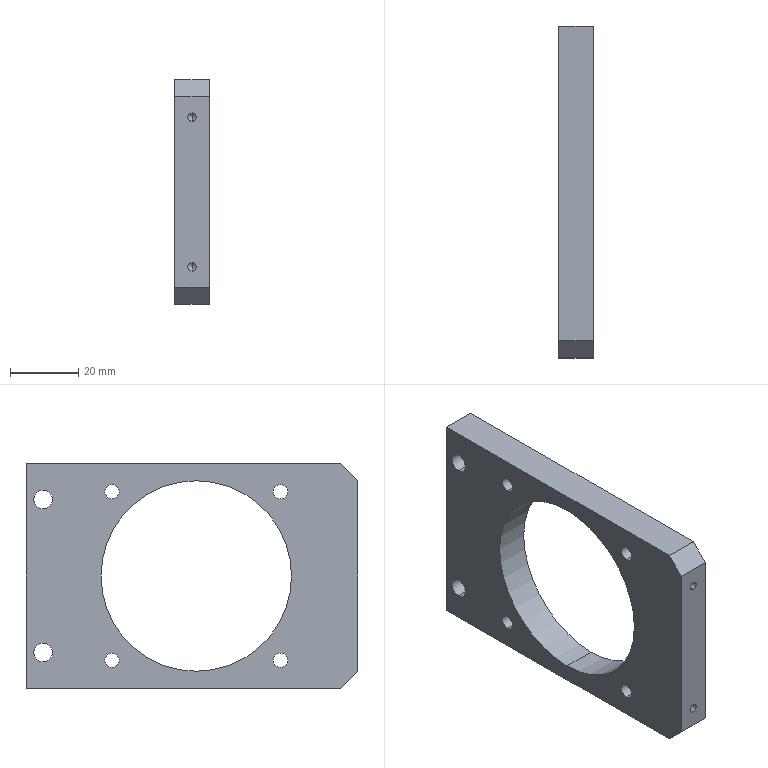Part | STEP file | 0243_221_Plate | 1 solid | 30 faces | box 10 x 97.5 x 66 mm | volume 38364 mm3 | cylinder 18 | plane 8 | cone 4 | commonest cylinder face diameters 4.2 x8 2.5 x4 5.5 x4 56 x2